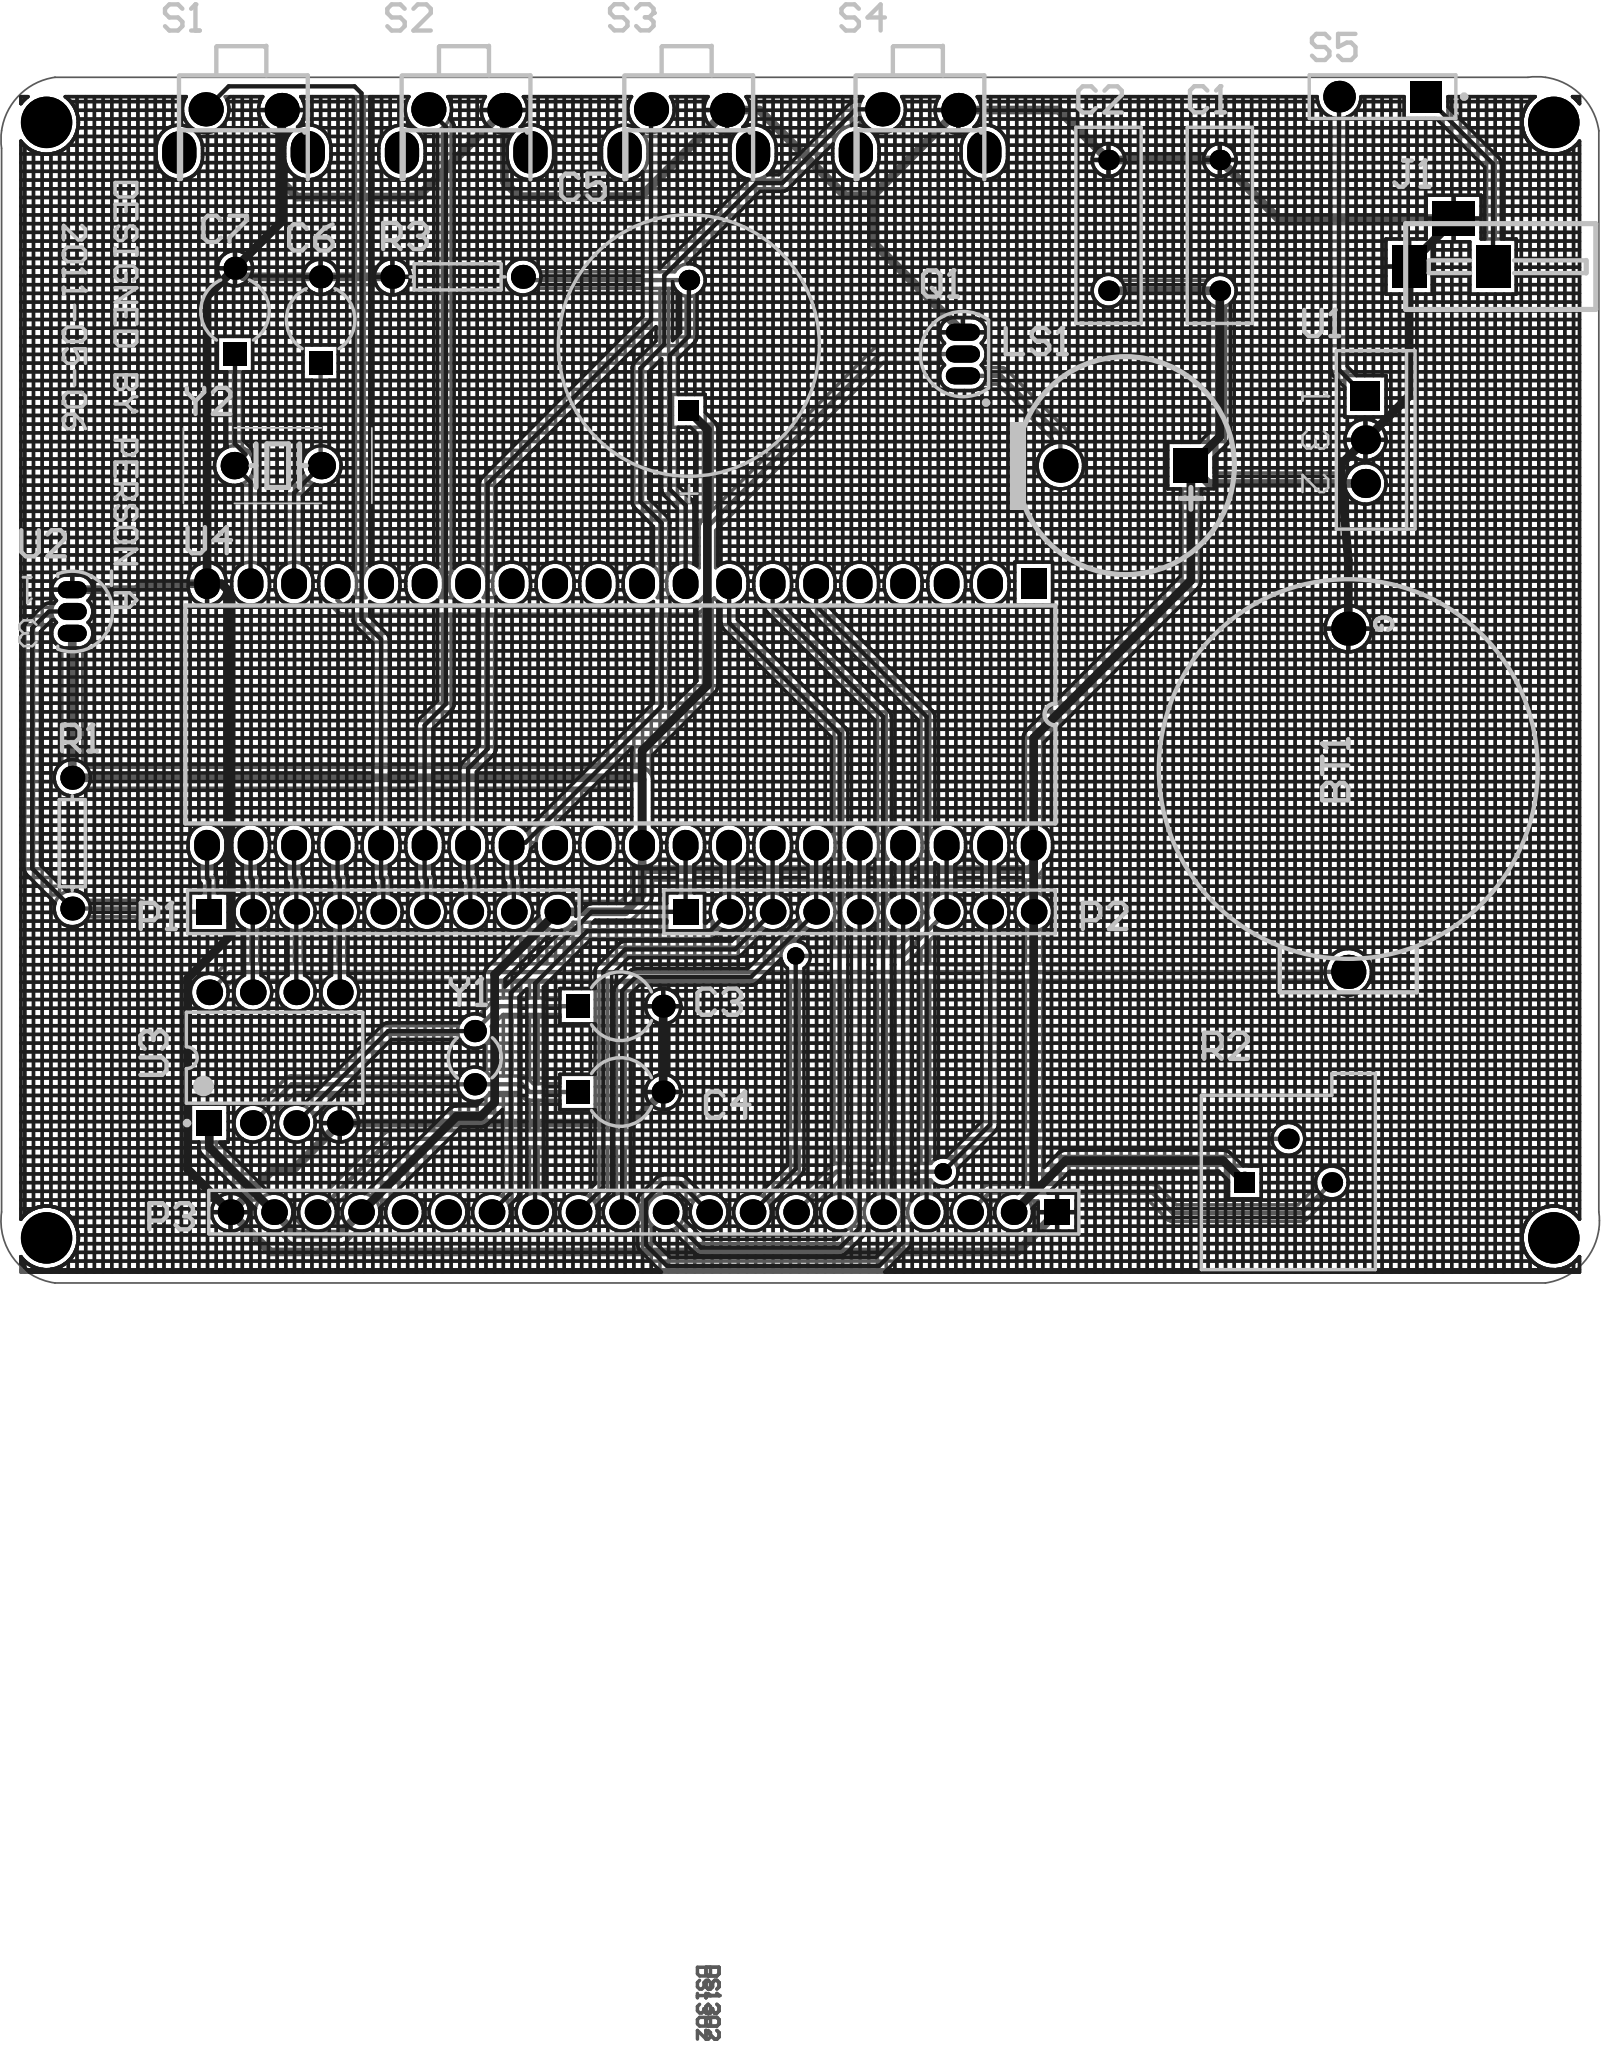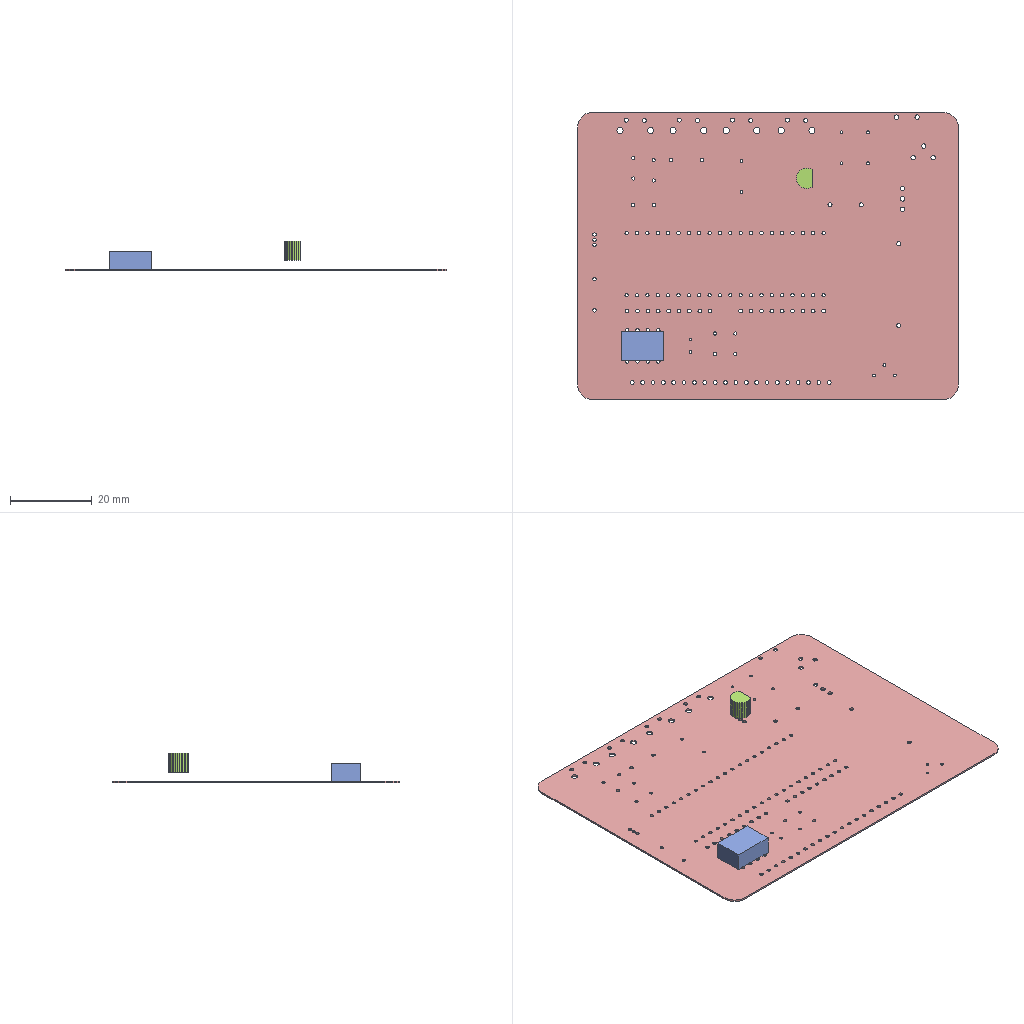Circuit board layout | Altium Designer | box 93.3 x 70.3 x 7.3 mm
Layer stack:
# Altium Designer layer stack of  (unit mm; dielectric type: 0 none, 1 core, 2 prepreg, 3 surface material)
index,name,kind,layer,copper_thickness_mm,dielectric_type,dielectric_thickness_mm,dielectric_material,dielectric_constant
0,Top Paste,other,,,,,,
1,Top Overlay,other,,,,,,
2,Top Solder,dielectric,,,3,0.0102,Solder Resist,3.5
3,Top Layer,copper,Top Layer,0.0356,,,,
4,Dielectric1,dielectric,,,0,0.32,FR-4,4.8
5,Bottom Layer,copper,Bottom Layer,0.0356,,,,
6,Bottom Solder,dielectric,,,3,0.0102,Solder Resist,3.5
7,Bottom Overlay,other,,,,,,
8,Bottom Paste,other,,,,,,
# drill layer pairs: low layer,high layer
drill_pair,Top Layer,Bottom Layer
Part placement:
Designator,Comment,Layer,Footprint,Center-X(mm),Center-Y(mm),Rotation
Y2,XTAL,TopLayer,XTAL2,16,-22.5,180
Y1,XTAL,TopLayer,R38,27.5,-57,360
U4,AT89S52-33PC,TopLayer,DIP40,36,-37,360
U3,DS1302,TopLayer,DIP8,15.81,-57,90
U2,DS1820,TopLayer,PR35,4,-31,180
U1,L7805ACV,TopLayer,TO220ABN,79.5,-21,270
S5,SW-SPST,TopLayer,SPST-2,80.5,-1,180
S4,SW-PB,TopLayer,SW4,53.5,-3,270
S3,SW-PB,TopLayer,SW4,40,-3,270
S2,SW-PB,TopLayer,SW4,27,-3,270
S1,SW-PB,TopLayer,SW4,14,-3,270
R3,Res1,TopLayer,AXIAL-0.3,26.5,-11.5,360
R2,RPot,TopLayer,VR4,75,-63,0
R1,Res1,TopLayer,AXIAL-0.3,4,-44.5,270
Q1,2N3906,TopLayer,TO-92A,56,-16,360
P3,Header 20,TopLayer,HDR1X20,37.37,-66,180
P2,Header 9,TopLayer,HDR1X9,49.97,-48.5,360
P1,Header 9,TopLayer,HDR1X9,22.16,-48.5,360
LS1,Bell,TopLayer,BELL,65.5,-22.5,90
J1,PWR2.5,TopLayer,DC,84.5,-9.5,360
C7,Cap2,TopLayer,CAPR5-4X5,13.5,-13.5,90
C6,Cap2,TopLayer,CAPR5-4X5,18.5,-14,90
C5,Cap Pol1,TopLayer,RB7.6-15,40,-15.5,270
C4,Cap2,TopLayer,CAPR5-4X5,36,-59,360
C3,Cap2,TopLayer,CAPR5-4X5,36,-54,0
C2,Cap,TopLayer,RAD-0.3,64.5,-8.5,270
C1,Cap,TopLayer,RAD-0.3,71,-8.5,270
BT1,Battery,TopLayer,3V电池,78.5,-42,360
Pad and via stacks:
# Altium Designer via and pad stacks of  (unit mm). Each distinct definition once, with the count of objects using it.
# via: kind,start_layer,end_layer,hole_mm,diameter_mm,mode(0 simple;1 top-mid-bottom;2 full stack),diameter_per_layer,count,example_net
# pad: kind,layer,hole_mm,hole_type(0 round;1 square;2 slot),plating,top_size,top_shape(1 round;2 rect;3 octagon;9 rounded rect),mid_size,bottom_size,mode,footprint,size_per_layer,count,example
pad,Multi-Layer,0.9,0,plated,1.5x1.5,2,1.5x1.5,1.5x1.5,0,HDR1X9,,2,P2.1
pad,Multi-Layer,0.9,0,plated,1.5x1.5,1,1.5x1.5,1.5x1.5,0,HDR1X9,,16,P2.3
pad,Multi-Layer,0.9,0,plated,1.5x1.5,2,1.5x1.5,1.5x1.5,0,HDR1X20,,1,P3.1
pad,Multi-Layer,0.9,0,plated,1.5x1.5,1,1.5x1.5,1.5x1.5,0,HDR1X20,,19,P3.2
pad,Multi-Layer,0.9,0,plated,1.5x1.5,2,1.5x1.5,1.5x1.5,0,DIP8,,1,U3.1
pad,Multi-Layer,0.9,0,plated,1.5x1.5,1,1.5x1.5,1.5x1.5,0,DIP8,,7,U3.2
pad,Multi-Layer,0.8,0,plated,1.35x1.35,1,1.35x1.35,1.35x1.35,0,CAPR5-4X5,,4,C3.2
pad,Multi-Layer,0.8,0,plated,1.35x1.35,2,1.35x1.35,1.35x1.35,0,CAPR5-4X5,,4,C3.1
pad,Multi-Layer,1,0,plated,2x2,1,2x2,2x2,0,BELL,,1,LS1.2
pad,Multi-Layer,1,0,plated,2x2,2,2x2,2x2,0,BELL,,1,LS1.1
pad,Multi-Layer,1,0,plated,2x2,1,2x2,2x2,0,3V\u00B5\u00E7\u00B3\u00D8,,2,BT1.1
pad,Multi-Layer,1.1,0,plated,1.7x1.7,1,1.7x1.7,1.7x1.7,0,TO220ABN,,2,U1.2
pad,Multi-Layer,1.1,0,plated,1.7x1.7,2,1.7x1.7,1.7x1.7,0,TO220ABN,,1,U1.1
pad,Multi-Layer,1.1,0,plated,1.85x1.85,2,1.85x1.85,1.85x1.85,0,SPST-2,,1,S5.1
pad,Multi-Layer,1.1,0,plated,1.85x1.85,1,1.85x1.85,1.85x1.85,0,SPST-2,,1,S5.2
pad,Multi-Layer,1.1,0,plated,2.5x2,2,2.5x2,2.5x2,0,DC,,2,J1.2
pad,Multi-Layer,1.1,0,plated,2x2.5,2,2x2.5,2x2.5,0,DC,,1,J1.3
pad,Multi-Layer,0.7,0,plated,1.2x1.2,1,1.2x1.2,1.2x1.2,0,RAD-0.3,,4,C2.2
pad,Multi-Layer,0.7,0,plated,1.2x1.2,2,1.2x1.2,1.2x1.2,0,VR4,,1,R2.1
pad,Multi-Layer,0.7,0,plated,1.2x1.2,1,1.2x1.2,1.2x1.2,0,VR4,,2,R2.3
pad,Multi-Layer,0.82,0,plated,1.8x1.5,1,1.8x1.5,1.8x1.5,0,DIP40,,39,U4.8
pad,Multi-Layer,0.82,0,plated,1.8x1.5,2,1.8x1.5,1.8x1.5,0,DIP40,,1,U4.1
pad,Multi-Layer,0.7,0,plated,1.2x1.2,2,1.2x1.2,1.2x1.2,0,RB7.6-15,,1,C5.1
pad,Multi-Layer,0.7,0,plated,1.2x1.2,1,1.2x1.2,1.2x1.2,0,RB7.6-15,,1,C5.2
pad,Multi-Layer,1,0,plated,2x2,1,2x2,2x2,0,SW4,,8,S1.1
pad,Multi-Layer,1.5,0,plated,2x2.5,1,2x2.5,2x2.5,0,SW4,,8,S1.0
pad,Multi-Layer,0.85,0,plated,1.4x1.4,1,1.4x1.4,1.4x1.4,0,AXIAL-0.3,,4,R3.2
pad,Multi-Layer,0.7,0,plated,1.3x1.3,1,1.3x1.3,1.3x1.3,0,R38,,2,Y1.1
pad,Multi-Layer,0.82,0,plated,1.6x1.6,1,1.6x1.6,1.6x1.6,0,XTAL2,,2,Y2.1
pad,Multi-Layer,0.8,0,plated,1.7x1,1,1.7x1,1.7x1,0,PR35,,3,U2.1
pad,Multi-Layer,0.9,0,plated,2x1,1,2x1,2x1,0,TO-92A,,3,Q1.3
via,Top Layer,Bottom Layer,3,3,0,,4,
via,Top Layer,Bottom Layer,0.4572,1.016,0,,2,NetP2_7
Copper pours:
name,layer,net,type(0 solid;1 hatched;2 none)
Top Overlay-No Net,Top Layer,GND,0
Top Overlay-No Net,Bottom Layer,GND,0
Design rules, without the lines most boards share:
# Altium Designer design rules of  (exported by Altium Designer, unit mm)
# columns: name | kind | enabled | priority | scope1 | scope2 | descriptor | typed fields (field=value)
power | 2 | enabled | 1 | InNet('VCC') Or InNet('GND') | All | Width Constraint (Min=8mil) (Max=30mil) (Preferred=20mil) (InNet('VCC') Or InNet('GND')) |
SilkToSilkClearance | 55 | enabled | 1 | All | All | Silk to Silk (Clearance=2mil) (All),(All) |
SilkscreenOverComponentPads | 54 | enabled | 1 | IsPad | All | Silk To Solder Mask (Clearance=0mil) (IsPad),(All) |
MinimumSolderMaskSliver | 53 | enabled | 1 | All | All | Minimum Solder Mask Sliver (Gap=2mil) (All),(All) |
HoleToHoleClearance | 52 | enabled | 1 | All | All | Hole To Hole Clearance (Gap=10mil) (All),(All) | gap=0.254
DiffPairsRouting | 51 | enabled | 1 | All | All | Differential Pairs Uncoupled Length using the Gap Constraints (Min=10mil) (Max=10mil) (Prefered=10mil)  and Width Constraints (Min=15mil) (Max=15mil) (Prefered=15mil) (All) |
HoleSize | 42 | enabled | 1 | All | All | Hole Size Constraint (Min=1mil) (Max=139.37mil) (All) |
RoutingTopology | 7 | enabled | 1 | All | All | Routing Topology Rule(Topology=Horizontal) (All) |
SolderMaskExpansion | 13 | enabled | 1 | All | All | Solder Mask Expansion (Expansion =4mil) (All) | expansion=0.1016
PasteMaskExpansion | 14 | enabled | 1 | All | All | Paste Mask Expansion (Expansion =0mil) (All) | expansion=0
RoutingVias | 11 | enabled | 1 | All | All | Routing Via (MinHoleWidth=38mil) (MaxHoleWidth=28mil) (PreferredHoleWidth=18mil) (MinWidth=60mil) (MaxWidth=50mil) (PreferedWidth=40mil) (All) | via_min_hole=0.9652 via_max_hole=0.7112 via_preferred_diameter=1.016 via_preferred_hole=0.4572
Width | 2 | enabled | 2 | All | All | Width Constraint (Min=5mil) (Max=20mil) (Preferred=10mil) (All) |
PolygonConnect | 20 | enabled | 1 | All | All | Polygon Connect Rule(Relief Connect )(Conductor Width=10mil) (Relief Angle=90 Angle) (Entries=4) (Air Gap Width=10mil) (All),(All) | connect_style(0=relief,1=direct,2=none)=0 relief_conductor_width=0.254 relief_entries=4
PlaneConnect | 6 | enabled | 1 | All | All | Power Plane Connect Rule(Relief Connect )(Expansion=20mil) (Conductor Width=10mil) (Air Gap=10mil) (Entries=4) (All) | relief_conductor_width=0.254 relief_entries=4 relief_expansion=0.508
Clearance | 0 | enabled | 1 | All | All | Clearance Constraint (Gap=10mil) (All),(All) | gap=0.254
Classes set for this board:
# Altium Designer classes of  (member kind: 0 net, 1 component, 2 from-to, 3 pad, 4 layer, 5 differential pair, 6 design channel, 7 polygon, 8 structure, 9 xSignal)
# columns: class name | member kind | superclass | members
Calender | 1 | no | BT1; C1; C2; C3; C4; C5; C6; C7; J1; LS1; P1; P2; P3; Q1; R1; R2; R3; S1; S2; S3; S4; S5; U1; U2; U3; U4; Y1; Y2;